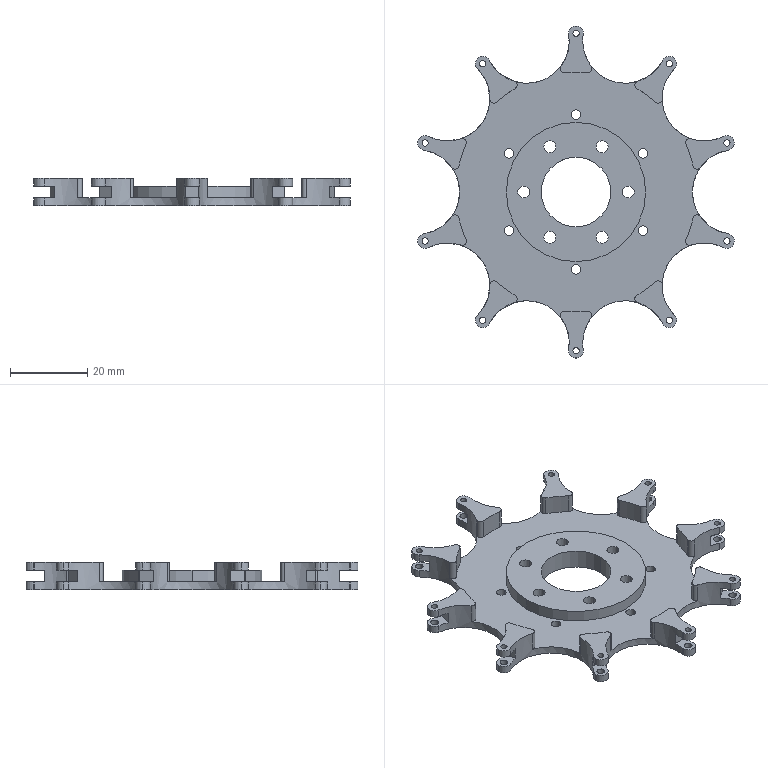Part | SolidWorks | features ICE 6, HoleWzd 2, Extrusion 1 | 1 solid | 202 faces | box 81.787 x 85.8 x 7 mm | volume 10881 mm3 | cylinder 159 | plane 43 | commonest cylinder face diameters 2 x48 3.8 x36 1.6 x20 21.855 x17 2.5 x12 3.1 x12